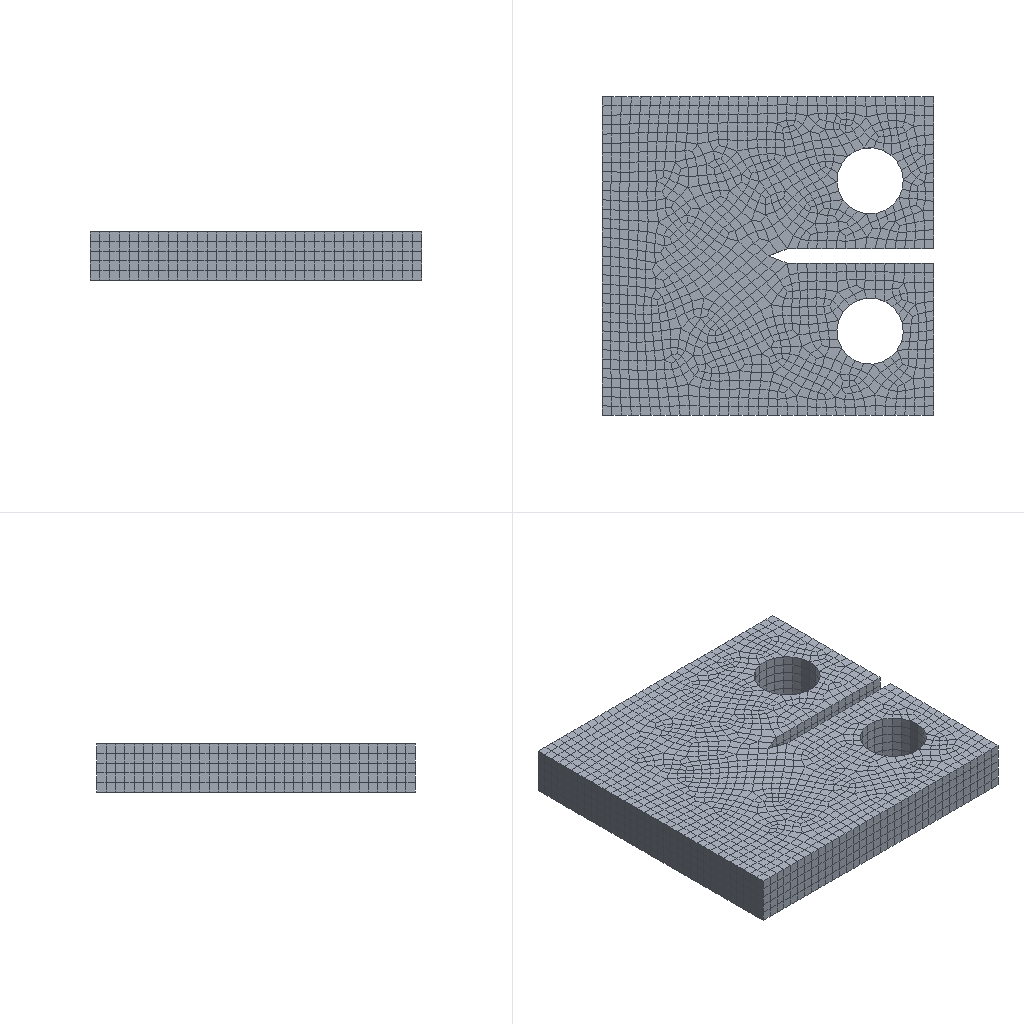Simulation study | abaqus
Set-up summary:
category,name,step,type,value,unit,region
solver,abaqus
solver,version,,,Abaqus/Standard 2020
units,not stated in the deck,,not stated
analysis,deck,,static,static
load_step,Step-1,Step-1,static
load_step,requested,,,1
mesh,nodes,,,8154
mesh,elements,,,6270
element_type,C3D8R,,solid,6270
load,load commands in deck,,count,2
bc,support commands in deck,,count,13
material,MATERIAL-1,,in results
check,setup vs results,,match,"per instance, exact: element labels, types and connectivity; labels of the nodes the elements use; coordinates of those nodes at SINGLE_PRECISION in 1 of 1 instance(s)"
Abaqus input file, long lists of numbers shortened:
*Heading
** Job name: Job-1 Model name: Model-1
** Generated by: Abaqus/CAE 2020
*Preprint, echo=NO, model=NO, history=NO, contact=NO
**
** PARTS
**
*Part, name=Part-1
*Node
      1,   34.38,          33.,           0.
      2,   34.38,          1.5,           0.
** (8152 more lines like these left out)
*Element, type=C3D8R
   1,  408,  247,  198,  270, 1767, 1606, 1557, 1629
   2,   53,  295,  296,   54, 1412, 1654, 1655, 1413
** (6268 more lines like these left out)
*Nset, nset=Set-1, generate
    1,  8154,     1
*Elset, elset=Set-1, generate
    1,  6270,     1
** Section: Section-1
*Solid Section, elset=Set-1, material=Material-1
,
*End Part
**
*Part, name=crack
*End Part
**
**
** ASSEMBLY
**
*Assembly, name=Assembly
**
*Instance, name=Part-1-1, part=Part-1
*End Instance
**
*Instance, name=crack-1, part=crack
         -5.,           0.,          -5.
         -5.,           0.,          -5., -6.,           0.,          -5., 90.
*End Instance
**
*Node
      1,   21.158,   15.568,           5.
*Node
      2,   21.158,  -15.568,           5.
*Nset, nset=Set-5, instance=Part-1-1
    9,   10,   11,  133,  134,  135,  136,  137,  138,  139,  140,  141,  142,  143,  144,  145
  146,  147,  148,  149,  150,  151,  152,  153,  154,  155,  156,  157,  158,  159,  160,  161
** (12 more lines like these left out)
*Elset, elset=Set-5, instance=Part-1-1
   13,   14,   27,  112,  114,  115,  126,  127,  129,  132,  133,  134,  135,  136,  139,  144
  145,  146,  147,  148,  149,  150,  153,  188,  190,  192,  194,  196,  198,  202,  207,  209
** (9 more lines like these left out)
*Nset, nset=Set-6
 1,
*Nset, nset=Set-7
 2,
*Nset, nset=m_Set-3
 1,
*Nset, nset=m_Set-4
 2,
*Nset, nset=_PickedSet6, internal, instance=Part-1-1, generate
    1,  8154,     1
*Elset, elset=_PickedSet6, internal, instance=Part-1-1, generate
    1,  6270,     1
*Elset, elset=_s_Surf-1_S6, internal, instance=Part-1-1
    5,   65,  221, 1259, 1319, 1475, 2513, 2573, 2729, 3767, 3827, 3983, 5021, 5081, 5237
*Elset, elset=_s_Surf-1_S4, internal, instance=Part-1-1
    8,   44,   59,  167,  177,  180,  229, 1262, 1298, 1313, 1421, 1431, 1434, 1483, 2516, 2552
 2567, 2675, 2685, 2688, 2737, 3770, 3806, 3821, 3929, 3939, 3942, 3991, 5024, 5060, 5075, 5183
** (1 more lines like these left out)
*Elset, elset=_s_Surf-1_S3, internal, instance=Part-1-1
   10,   30,   46,  176,  179, 1264, 1284, 1300, 1430, 1433, 2518, 2538, 2554, 2684, 2687, 3772
 3792, 3808, 3938, 3941, 5026, 5046, 5062, 5192, 5195
*Elset, elset=_s_Surf-1_S5, internal, instance=Part-1-1
  161,  182,  211,  223,  235,  247,  254, 1415, 1436, 1465, 1477, 1489, 1501, 1508, 2669, 2690
 2719, 2731, 2743, 2755, 2762, 3923, 3944, 3973, 3985, 3997, 4009, 4016, 5177, 5198, 5227, 5239
** (1 more lines like these left out)
*Surface, type=ELEMENT, name=s_Surf-1
_s_Surf-1_S6, S6
_s_Surf-1_S4, S4
_s_Surf-1_S3, S3
_s_Surf-1_S5, S5
*Elset, elset=_s_Surf-2_S5, internal, instance=Part-1-1
   16,   71,   80,   98,  213,  226,  231, 1270, 1325, 1334, 1352, 1467, 1480, 1485, 2524, 2579
 2588, 2606, 2721, 2734, 2739, 3778, 3833, 3842, 3860, 3975, 3988, 3993, 5032, 5087, 5096, 5114
** (1 more lines like these left out)
*Elset, elset=_s_Surf-2_S6, internal, instance=Part-1-1
   19,   21,   41,   79,  100,  105,  246, 1273, 1275, 1295, 1333, 1354, 1359, 1500, 2527, 2529
 2549, 2587, 2608, 2613, 2754, 3781, 3783, 3803, 3841, 3862, 3867, 4008, 5035, 5037, 5057, 5095
** (1 more lines like these left out)
*Elset, elset=_s_Surf-2_S4, internal, instance=Part-1-1
   92,  107,  216,  220,  233, 1346, 1361, 1470, 1474, 1487, 2600, 2615, 2724, 2728, 2741, 3854
 3869, 3978, 3982, 3995, 5108, 5123, 5232, 5236, 5249
*Elset, elset=_s_Surf-2_S3, internal, instance=Part-1-1
   93,   96,  102, 1347, 1350, 1356, 2601, 2604, 2610, 3855, 3858, 3864, 5109, 5112, 5118
*Surface, type=ELEMENT, name=s_Surf-2
_s_Surf-2_S5, S5
_s_Surf-2_S6, S6
_s_Surf-2_S4, S4
_s_Surf-2_S3, S3
** Constraint: Constraint-1
*Coupling, constraint name=Constraint-1, ref node=m_Set-3, surface=s_Surf-1
*Kinematic
** Constraint: Constraint-2
*Coupling, constraint name=Constraint-2, ref node=m_Set-4, surface=s_Surf-2
*Kinematic
*Enrichment, name=Crack-1, type=PROPAGATION CRACK, elset=_PickedSet6
*End Assembly
*Amplitude, name=u1, definition=PERIODIC
1,           125.6,              0.,              0.
             1.,              0.
*Amplitude, name=u2, definition=PERIODIC
1,           125.6,              0.,              0.
             1.,              0.
**
** MATERIALS
**
*Material, name=Material-1
*Damage Initiation, criterion=MAXPS
800.,
*Damage Evolution, type=DISPLACEMENT
 1e-06,
*Elastic
210000., 0.3
*Initial Conditions, type=ENRICHMENT
Part-1-1.384, 1,Crack-1, 0.01594, 1.915
Part-1-1.384, 2,Crack-1, -1.339, 0.354
Part-1-1.384, 3,Crack-1, 1e-06, -1.
Part-1-1.384, 4,Crack-1, 1.395, 0.3713
Part-1-1.384, 5,Crack-1, 0.01594, 1.915
Part-1-1.384, 6,Crack-1, -1.339, 0.354
Part-1-1.384, 7,Crack-1, 1e-06, -1.
Part-1-1.384, 8,Crack-1, 1.395, 0.3713
Part-1-1.164, 1,Crack-1, 0.01594, 1.915
Part-1-1.164, 2,Crack-1, -1.339, 0.354
Part-1-1.164, 3,Crack-1, 1e-06, -1.
Part-1-1.164, 4,Crack-1, 1.395, 0.3713
Part-1-1.164, 5,Crack-1, 0.01594, 1.915
Part-1-1.164, 6,Crack-1, -1.339, 0.354
Part-1-1.164, 7,Crack-1, 1e-06, -1.
Part-1-1.164, 8,Crack-1, 1.395, 0.3713
Part-1-1.289, 1,Crack-1, 0.01594, 1.915
Part-1-1.289, 2,Crack-1, -1.339, 0.354
Part-1-1.289, 3,Crack-1, 1e-06, -1.
Part-1-1.289, 4,Crack-1, 1.395, 0.3713
Part-1-1.289, 5,Crack-1, 0.01594, 1.915
Part-1-1.289, 6,Crack-1, -1.339, 0.354
Part-1-1.289, 7,Crack-1, 1e-06, -1.
Part-1-1.289, 8,Crack-1, 1.395, 0.3713
Part-1-1.415, 1,Crack-1, 0.01594, 1.915
Part-1-1.415, 2,Crack-1, -1.339, 0.354
Part-1-1.415, 3,Crack-1, 1e-06, -1.
Part-1-1.415, 4,Crack-1, 1.395, 0.3713
Part-1-1.415, 5,Crack-1, 0.01594, 1.915
Part-1-1.415, 6,Crack-1, -1.339, 0.354
Part-1-1.415, 7,Crack-1, 1e-06, -1.
Part-1-1.415, 8,Crack-1, 1.395, 0.3713
Part-1-1.54, 1,Crack-1, 0.01594, 1.915
Part-1-1.54, 2,Crack-1, -1.339, 0.354
Part-1-1.54, 3,Crack-1, 1e-06, -1.
Part-1-1.54, 4,Crack-1, 1.395, 0.3713
Part-1-1.54, 5,Crack-1, 0.01594, 1.915
Part-1-1.54, 6,Crack-1, -1.339, 0.354
Part-1-1.54, 7,Crack-1, 1e-06, -1.
Part-1-1.54, 8,Crack-1, 1.395, 0.3713
** (40 more lines like these left out)
** ----------------------------------------------------------------
**
** STEP: Step-1
**
*Step, name=Step-1, nlgeom=YES, inc=1000
*Static, stabilize=0.0002, allsdtol=0.05, continue=NO
0.01, 1., 1e-05, 1.
**
** BOUNDARY CONDITIONS
**
** Name: BC-1 Type: 对称/反对称/完全固定
*Boundary
Set-5, ENCASTRE
** Name: [REDACTED]
*Boundary, amplitude=u1
Set-6, 1, 1
Set-6, 2, 2, 0.2
Set-6, 3, 3
Set-6, 4, 4
Set-6, 5, 5
Set-6, 6, 6
** Name: [REDACTED]
*Boundary, amplitude=u2
Set-7, 1, 1
Set-7, 2, 2, -0.2
Set-7, 3, 3
Set-7, 4, 4
Set-7, 5, 5
Set-7, 6, 6
**
** CONTROLS
**
*Controls, reset
*Controls, parameters=time incrementation
, , , , , , , 20, , ,
**
** OUTPUT REQUESTS
**
*Restart, write, frequency=0
**
** FIELD OUTPUT: F-Output-1
**
*Output, field
*Node Output
CF, PHILSM, PSILSM, RF, RM, RT, TF, U
UR, UT, V, VR, VT
*Element Output, directions=YES
E, ENER, ENRRTXFEM, ER, LE, LOADSXFEM, MISES, MISESMAX, MISESONLY, PE, PEEQ, PEEQMAX, PEEQT, PEMAG, S, SDEG
SF, SSAVG, STATUS, STATUSXFEM, VEEQ
*Contact Output
CDISP, CRSTS, CSTATUS, CSTRESS, DBT, ENRRT, PPRESS
**
** HISTORY OUTPUT: H-Output-3
**
*Output, history
*Contact Output
ENRRT11, ENRRT12, ENRRT13
**
** HISTORY OUTPUT: H-Output-1
**
*Output, history, variable=PRESELECT
*End Step
Results summary:
result,step,,completed,increments=70 time=1.0/1.0
result,analysis,,,static
result,last_loadstep,,,1
result,primary field,,,U
result,reaction total,,FX,1.111,model units
result,reaction total,,FY,-1.391,model units
result,reaction total,,FZ,-0.001422,model units